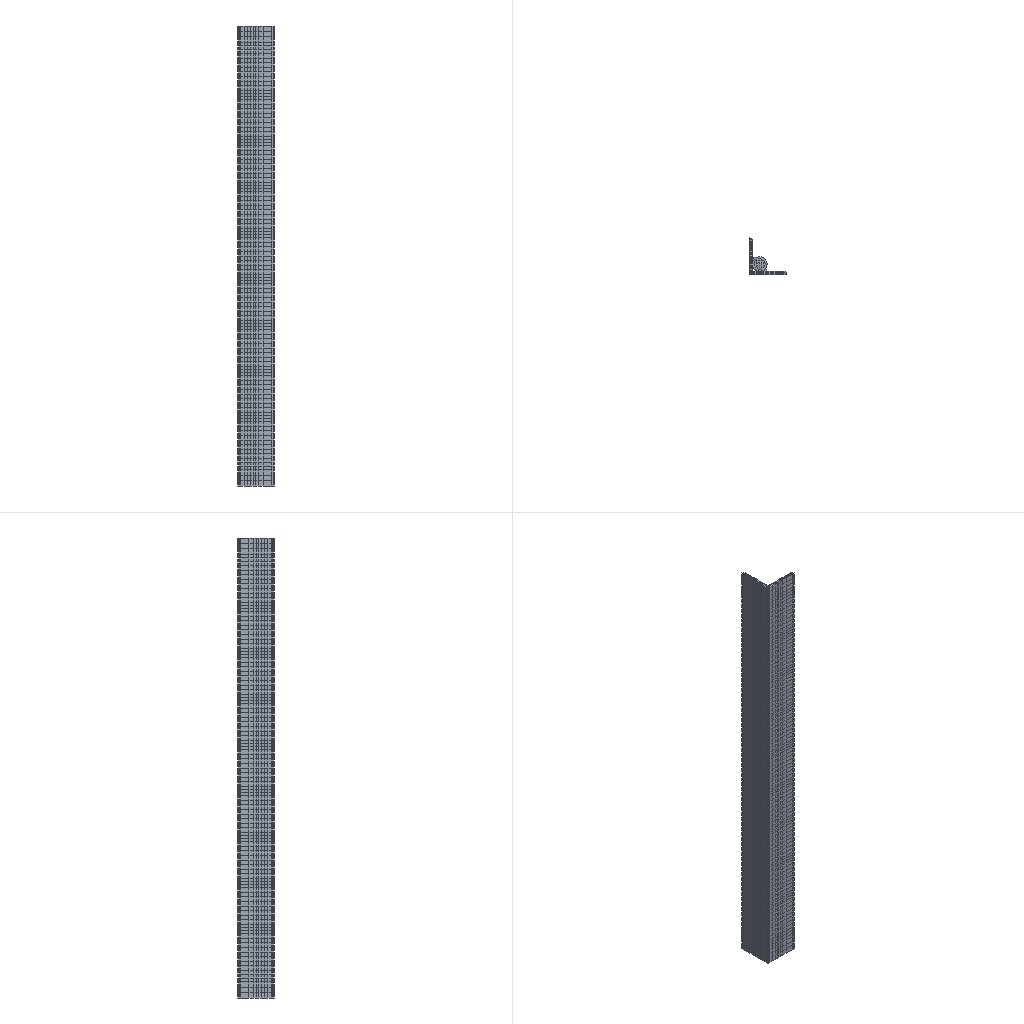Simulation study | abaqus
Set-up summary:
category,name,step,type,value,unit,region
solver,abaqus
solver,version,,,Abaqus/Explicit 3DEXPERIENCE R2017x
units,not stated in the deck,,not stated
analysis,deck,,transient,transient
load_step,Step-2,Step-2,transient
load_step,requested,,,1
mesh,nodes,,,15766
mesh,elements,,,12256
element_type,C3D8R,,solid,12256
load,load commands in deck,,count,1
bc,support commands in deck,,count,15
material,Q235,,in results
check,setup vs results,,match,"per instance, exact: element labels, types and connectivity; labels of the nodes the elements use; coordinates not compared"
Abaqus input file, long lists of numbers shortened:
*Heading
** Job name: Job-final Model name: yawan
** Generated by: Abaqus/CAE 2017
*Preprint, echo=NO, model=NO, history=NO, contact=NO
**
** PARTS
**
*Part, name=PART-1
*Node
      1, 0.002595, 0.005076, -0.36
      2, 0.002595, -0.0009244, -0.36
** (15764 more lines like these left out)
*Element, type=C3D8R
    1,   716,  4724, 11552,  4720,     1,   699,  4712,   706
    2,  4724,  4725, 11553, 11552,   699,   700,  4713,  4712
** (12254 more lines like these left out)
*Nset, nset=SET-T, generate
     1,  15766,      1
*Elset, elset=SET-T, generate
     1,  12256,      1
** Section: Section-1-SET-T
*Solid Section, elset=SET-T, material=Q235
,
*End Part
**
**
** ASSEMBLY
**
*Assembly, name=Assembly
**
*Instance, name=PART-1-1, part=PART-1
*End Instance
**
*Node
      1, 0.002795, 0.02128,          0.5
      2, 0.002795, 0.02128,         -0.5
*Nset, nset=Set-13
 2,
*Nset, nset=Set-14
 1,
*Elset, elset=Set-15, instance=PART-1-1, generate
     1,  12256,      1
*Nset, nset=Set-16, instance=PART-1-1, generate
     1,  15766,      1
*Nset, nset=Set-16
 1, 2
*Nset, nset=Set-17, instance=PART-1-1
     2,     3,     6,     7,    10,    11,    13,    16,   115,   116,   118,   119,   123,   124,   126,   127
   131,   132,   134,   137,   140,   141,   142,   145,   146,   149,   150,   153,   154,   156,   159,   162
** (94 more lines like these left out)
*Elset, elset=Set-22, instance=PART-1-1, generate
     1,  12256,      1
*Elset, elset=Set-23, instance=PART-1-1, generate
     1,  12256,      1
*Nset, nset=Set-24
 1,
*Nset, nset=Set-25
 1,
*Nset, nset=m_Set-17
 1,
*Nset, nset=m_Set-18
 2,
*Nset, nset=m_Set-19
 1,
*Nset, nset=m_Set-20
 2,
*Nset, nset=s_Set-20, instance=PART-1-1
   116,   117,   119,   120,   144,   145,   350,   351,   352,   353,   354,   355,   426,   427,   475,   476
   495,   496,   548,   549,   572,   657,  1088,  1089,  1096,  1097,  1100,  1102,  1182,  1183,  2346,  2351
** (4 more lines like these left out)
*Nset, nset=s_Set-21, instance=PART-1-1
   136,   137,   139,   140,   154,   155,   178,   179,   316,   317,   318,   319,   356,   357,   393,   394
   435,   436,   547,   570,   574,   658,  1162,  1163,  1170,  1171,  1174,  1176,  1214,  1215,  1282,  1283
** (4 more lines like these left out)
*Elset, elset=_SURF-1_S2, internal, instance=PART-1-1
 7817, 7818, 7819, 7820, 7821, 9959, 9960, 9961, 9962, 9963, 9964, 9965, 9966, 9967
*Elset, elset=_SURF-1_S3, internal, instance=PART-1-1
 8327, 8328, 8331
*Elset, elset=_SURF-1_S4, internal, instance=PART-1-1
 2524, 2527, 2530, 8325, 8326
*Elset, elset=_SURF-1_S5, internal, instance=PART-1-1
  457,  458,  459,  466,  467,  468,  559,  560,  561, 4244, 4245, 4246, 4253, 4254, 4255, 4262
 4263, 4264, 5003, 5004, 5005, 5012, 5013, 5014, 6077, 6078, 6079, 6086, 6087, 6088, 6095, 6096
** (1 more lines like these left out)
*Elset, elset=_SURF-1_S6, internal, instance=PART-1-1, generate
 2504,  2519,     3
*Elset, elset=_SURF-2_S2, internal, instance=PART-1-1, generate
 9986,  9994,     1
*Elset, elset=_SURF-2_S3, internal, instance=PART-1-1
 8295, 8300, 8301, 8337, 8338, 8343, 8345
*Elset, elset=_SURF-2_S4, internal, instance=PART-1-1
 8293, 8294, 8342
*Elset, elset=_SURF-2_S5, internal, instance=PART-1-1
  541,  542,  543,  550,  551,  552,  601,  602,  603,  694,  695,  696,  703,  704,  705,  712
  713,  714, 2645, 2646, 2647, 2654, 2655, 2656, 3455, 3456, 3457, 3464, 3465, 3466, 3473, 3474
** (1 more lines like these left out)
*Elset, elset=_SURF-2_S6, internal, instance=PART-1-1, generate
 2135,  2141,     3
*Elset, elset=_SURF-1_S5_1, internal, instance=PART-1-1
  457,  458,  459,  466,  467,  468,  559,  560,  561, 4244, 4245, 4246, 4253, 4254, 4255, 4262
 4263, 4264, 5003, 5004, 5005, 5012, 5013, 5014, 6077, 6078, 6079, 6086, 6087, 6088, 6095, 6096
** (1 more lines like these left out)
*Elset, elset=_SURF-1_S4_1, internal, instance=PART-1-1
 2524, 2527, 2530, 8325, 8326
*Elset, elset=_SURF-1_S6_1, internal, instance=PART-1-1, generate
 2504,  2519,     3
*Elset, elset=_SURF-1_S2_1, internal, instance=PART-1-1
 7817, 7818, 7819, 7820, 7821, 9959, 9960, 9961, 9962, 9963, 9964, 9965, 9966, 9967
*Elset, elset=_SURF-1_S3_1, internal, instance=PART-1-1
 8327, 8328, 8331
*Surface, type=ELEMENT, name=SURF-1
_SURF-1_S5_1, S5
_SURF-1_S4_1, S4
_SURF-1_S6_1, S6
_SURF-1_S2_1, S2
_SURF-1_S3_1, S3
*Elset, elset=_SURF-2_S5_1, internal, instance=PART-1-1
  541,  542,  543,  550,  551,  552,  601,  602,  603,  694,  695,  696,  703,  704,  705,  712
  713,  714, 2645, 2646, 2647, 2654, 2655, 2656, 3455, 3456, 3457, 3464, 3465, 3466, 3473, 3474
** (1 more lines like these left out)
*Elset, elset=_SURF-2_S6_1, internal, instance=PART-1-1, generate
 2135,  2141,     3
*Elset, elset=_SURF-2_S4_1, internal, instance=PART-1-1
 8293, 8294, 8342
*Elset, elset=_SURF-2_S2_1, internal, instance=PART-1-1, generate
 9986,  9994,     1
*Elset, elset=_SURF-2_S3_1, internal, instance=PART-1-1
 8295, 8300, 8301, 8337, 8338, 8343, 8345
*Surface, type=ELEMENT, name=SURF-2
_SURF-2_S5_1, S5
_SURF-2_S6_1, S6
_SURF-2_S4_1, S4
_SURF-2_S2_1, S2
_SURF-2_S3_1, S3
*Elset, elset=_Surf-3_S1, internal, instance=PART-1-1
 1254, 1255, 1256, 1257, 1435, 1436, 1437, 1438, 1439, 1440, 1441, 1442, 1443, 1444, 2141, 2142
 2143, 2176, 2177, 2178, 2179, 2180, 2181, 2182, 2183, 2184, 2185, 2186, 2187, 2188, 2189, 2190
** (11 more lines like these left out)
*Elset, elset=_Surf-3_S2, internal, instance=PART-1-1
   865,   866,   867,   868,   869,   870,   871,   872,   873,   874,   875,   876,  1036,  1037,  1038,  1039
  1040,  1041,  1076,  1077,  1078,  1079,  1084,  1085,  1086,  1087,  1088,  1089,  1090,  1091,  1092,  1093
** (35 more lines like these left out)
*Elset, elset=_Surf-3_S3, internal, instance=PART-1-1
   823,   824,   825,   832,   833,   834,   841,   842,   843,   873,   874,   893,   894,   897,   898,   928
   929,   932,   933,   952,   953,   954,   958,   959,   960,   976,   977,   980,   981,   984,   985,  1004
** (66 more lines like these left out)
*Elset, elset=_Surf-3_S4, internal, instance=PART-1-1
     3,     6,     9,    12,    15,    18,    21,    24,    27,    30,    33,    36,    39,    42,    45,    48
    51,    54,    57,    60,    63,    66,    69,    72,    75,    78,    81,    84,    87,    90,    93,    96
** (172 more lines like these left out)
*Elset, elset=_Surf-3_S5, internal, instance=PART-1-1
   457,   458,   459,   466,   467,   468,   541,   542,   543,   550,   551,   552,   559,   560,   561,   601
   602,   603,   694,   695,   696,   703,   704,   705,   712,   713,   714,   829,   830,   831,   838,   839
** (33 more lines like these left out)
*Elset, elset=_Surf-3_S6, internal, instance=PART-1-1
     1,     4,     7,    10,    13,    16,    19,    22,    25,    28,    31,    34,    37,    40,    43,    46
    49,    52,    55,    58,    61,    64,    67,    70,    73,    76,    79,    82,    85,    88,    91,    94
** (119 more lines like these left out)
*Surface, type=ELEMENT, name=Surf-3
_Surf-3_S1, S1
_Surf-3_S2, S2
_Surf-3_S4, S4
_Surf-3_S6, S6
_Surf-3_S3, S3
_Surf-3_S5, S5
*Elset, elset=_Surf-4_S1, internal, instance=PART-1-1
 1254, 1255, 1256, 1257, 1435, 1436, 1437, 1438, 1439, 1440, 1441, 1442, 1443, 1444, 2141, 2142
 2143, 2176, 2177, 2178, 2179, 2180, 2181, 2182, 2183, 2184, 2185, 2186, 2187, 2188, 2189, 2190
** (11 more lines like these left out)
*Elset, elset=_Surf-4_S2, internal, instance=PART-1-1
   865,   866,   867,   868,   869,   870,   871,   872,   873,   874,   875,   876,  1036,  1037,  1038,  1039
  1040,  1041,  1076,  1077,  1078,  1079,  1084,  1085,  1086,  1087,  1088,  1089,  1090,  1091,  1092,  1093
** (35 more lines like these left out)
*Elset, elset=_Surf-4_S3, internal, instance=PART-1-1
   823,   824,   825,   832,   833,   834,   841,   842,   843,   873,   874,   893,   894,   897,   898,   928
   929,   932,   933,   952,   953,   954,   958,   959,   960,   976,   977,   980,   981,   984,   985,  1004
** (66 more lines like these left out)
*Elset, elset=_Surf-4_S4, internal, instance=PART-1-1
     3,     6,     9,    12,    15,    18,    21,    24,    27,    30,    33,    36,    39,    42,    45,    48
    51,    54,    57,    60,    63,    66,    69,    72,    75,    78,    81,    84,    87,    90,    93,    96
** (172 more lines like these left out)
*Elset, elset=_Surf-4_S5, internal, instance=PART-1-1
   457,   458,   459,   466,   467,   468,   541,   542,   543,   550,   551,   552,   559,   560,   561,   601
   602,   603,   694,   695,   696,   703,   704,   705,   712,   713,   714,   829,   830,   831,   838,   839
** (33 more lines like these left out)
*Elset, elset=_Surf-4_S6, internal, instance=PART-1-1
     1,     4,     7,    10,    13,    16,    19,    22,    25,    28,    31,    34,    37,    40,    43,    46
    49,    52,    55,    58,    61,    64,    67,    70,    73,    76,    79,    82,    85,    88,    91,    94
** (119 more lines like these left out)
*Surface, type=ELEMENT, name=Surf-4
_Surf-4_S1, S1
_Surf-4_S2, S2
_Surf-4_S4, S4
_Surf-4_S6, S6
_Surf-4_S3, S3
_Surf-4_S5, S5
*Elset, elset=_Surf-9_S1, internal, instance=PART-1-1
 1254, 1255, 1256, 1257, 1435, 1436, 1437, 1438, 1439, 1440, 1441, 1442, 1443, 1444, 2141, 2142
 2143, 2176, 2177, 2178, 2179, 2180, 2181, 2182, 2183, 2184, 2185, 2186, 2187, 2188, 2189, 2190
** (11 more lines like these left out)
*Elset, elset=_Surf-9_S2, internal, instance=PART-1-1
   865,   866,   867,   868,   869,   870,   871,   872,   873,   874,   875,   876,  1036,  1037,  1038,  1039
  1040,  1041,  1076,  1077,  1078,  1079,  1084,  1085,  1086,  1087,  1088,  1089,  1090,  1091,  1092,  1093
** (35 more lines like these left out)
*Elset, elset=_Surf-9_S3, internal, instance=PART-1-1
   823,   824,   825,   832,   833,   834,   841,   842,   843,   873,   874,   893,   894,   897,   898,   928
   929,   932,   933,   952,   953,   954,   958,   959,   960,   976,   977,   980,   981,   984,   985,  1004
** (66 more lines like these left out)
*Elset, elset=_Surf-9_S4, internal, instance=PART-1-1
     3,     6,     9,    12,    15,    18,    21,    24,    27,    30,    33,    36,    39,    42,    45,    48
    51,    54,    57,    60,    63,    66,    69,    72,    75,    78,    81,    84,    87,    90,    93,    96
** (172 more lines like these left out)
*Elset, elset=_Surf-9_S5, internal, instance=PART-1-1
   457,   458,   459,   466,   467,   468,   541,   542,   543,   550,   551,   552,   559,   560,   561,   601
   602,   603,   694,   695,   696,   703,   704,   705,   712,   713,   714,   829,   830,   831,   838,   839
** (33 more lines like these left out)
*Elset, elset=_Surf-9_S6, internal, instance=PART-1-1
     1,     4,     7,    10,    13,    16,    19,    22,    25,    28,    31,    34,    37,    40,    43,    46
    49,    52,    55,    58,    61,    64,    67,    70,    73,    76,    79,    82,    85,    88,    91,    94
** (119 more lines like these left out)
*Surface, type=ELEMENT, name=Surf-9
_Surf-9_S1, S1
_Surf-9_S2, S2
_Surf-9_S4, S4
_Surf-9_S6, S6
_Surf-9_S3, S3
_Surf-9_S5, S5
*Elset, elset=_Surf-10_S1, internal, instance=PART-1-1
 1254, 1255, 1256, 1257, 1435, 1436, 1437, 1438, 1439, 1440, 1441, 1442, 1443, 1444, 2141, 2142
 2143, 2176, 2177, 2178, 2179, 2180, 2181, 2182, 2183, 2184, 2185, 2186, 2187, 2188, 2189, 2190
** (11 more lines like these left out)
*Elset, elset=_Surf-10_S2, internal, instance=PART-1-1
   865,   866,   867,   868,   869,   870,   871,   872,   873,   874,   875,   876,  1036,  1037,  1038,  1039
  1040,  1041,  1076,  1077,  1078,  1079,  1084,  1085,  1086,  1087,  1088,  1089,  1090,  1091,  1092,  1093
** (35 more lines like these left out)
*Elset, elset=_Surf-10_S3, internal, instance=PART-1-1
   823,   824,   825,   832,   833,   834,   841,   842,   843,   873,   874,   893,   894,   897,   898,   928
   929,   932,   933,   952,   953,   954,   958,   959,   960,   976,   977,   980,   981,   984,   985,  1004
** (66 more lines like these left out)
*Elset, elset=_Surf-10_S4, internal, instance=PART-1-1
     3,     6,     9,    12,    15,    18,    21,    24,    27,    30,    33,    36,    39,    42,    45,    48
    51,    54,    57,    60,    63,    66,    69,    72,    75,    78,    81,    84,    87,    90,    93,    96
** (172 more lines like these left out)
*Elset, elset=_Surf-10_S5, internal, instance=PART-1-1
   457,   458,   459,   466,   467,   468,   541,   542,   543,   550,   551,   552,   559,   560,   561,   601
   602,   603,   694,   695,   696,   703,   704,   705,   712,   713,   714,   829,   830,   831,   838,   839
** (33 more lines like these left out)
*Elset, elset=_Surf-10_S6, internal, instance=PART-1-1
     1,     4,     7,    10,    13,    16,    19,    22,    25,    28,    31,    34,    37,    40,    43,    46
    49,    52,    55,    58,    61,    64,    67,    70,    73,    76,    79,    82,    85,    88,    91,    94
** (119 more lines like these left out)
*Surface, type=ELEMENT, name=Surf-10
_Surf-10_S1, S1
_Surf-10_S2, S2
_Surf-10_S4, S4
_Surf-10_S6, S6
_Surf-10_S3, S3
_Surf-10_S5, S5
*Elset, elset=_s_Surf-5_S2, internal, instance=PART-1-1
 7817, 7818, 7819, 7820, 7821, 9959, 9960, 9961, 9962, 9963, 9964, 9965, 9966, 9967
*Elset, elset=_s_Surf-5_S3, internal, instance=PART-1-1
 8327, 8328, 8331
*Elset, elset=_s_Surf-5_S4, internal, instance=PART-1-1
 2524, 2527, 2530, 8325, 8326
*Elset, elset=_s_Surf-5_S5, internal, instance=PART-1-1
  457,  458,  459,  466,  467,  468,  559,  560,  561, 4244, 4245, 4246, 4253, 4254, 4255, 4262
 4263, 4264, 5003, 5004, 5005, 5012, 5013, 5014, 6077, 6078, 6079, 6086, 6087, 6088, 6095, 6096
** (1 more lines like these left out)
*Elset, elset=_s_Surf-5_S6, internal, instance=PART-1-1, generate
 2504,  2519,     3
*Surface, type=ELEMENT, name=s_Surf-5
_s_Surf-5_S2, S2
_s_Surf-5_S3, S3
_s_Surf-5_S4, S4
_s_Surf-5_S6, S6
_s_Surf-5_S5, S5
*Elset, elset=_s_Surf-6_S2, internal, instance=PART-1-1, generate
 9986,  9994,     1
*Elset, elset=_s_Surf-6_S3, internal, instance=PART-1-1
 8295, 8300, 8301, 8337, 8338, 8343, 8345
*Elset, elset=_s_Surf-6_S4, internal, instance=PART-1-1
 8293, 8294, 8342
*Elset, elset=_s_Surf-6_S5, internal, instance=PART-1-1
  541,  542,  543,  550,  551,  552,  601,  602,  603,  694,  695,  696,  703,  704,  705,  712
  713,  714, 2645, 2646, 2647, 2654, 2655, 2656, 3455, 3456, 3457, 3464, 3465, 3466, 3473, 3474
** (1 more lines like these left out)
*Elset, elset=_s_Surf-6_S6, internal, instance=PART-1-1, generate
 2135,  2141,     3
*Surface, type=ELEMENT, name=s_Surf-6
_s_Surf-6_S2, S2
_s_Surf-6_S3, S3
_s_Surf-6_S4, S4
_s_Surf-6_S6, S6
_s_Surf-6_S5, S5
*Elset, elset=_s_Surf-7_S2, internal, instance=PART-1-1
 7817, 7818, 7819, 7820, 7821, 9959, 9960, 9961, 9962, 9963, 9964, 9965, 9966, 9967
*Elset, elset=_s_Surf-7_S3, internal, instance=PART-1-1
 8327, 8328, 8331
*Elset, elset=_s_Surf-7_S4, internal, instance=PART-1-1
 2524, 2527, 2530, 8325, 8326
*Elset, elset=_s_Surf-7_S5, internal, instance=PART-1-1
  457,  458,  459,  466,  467,  468,  559,  560,  561, 4244, 4245, 4246, 4253, 4254, 4255, 4262
 4263, 4264, 5003, 5004, 5005, 5012, 5013, 5014, 6077, 6078, 6079, 6086, 6087, 6088, 6095, 6096
** (1 more lines like these left out)
*Elset, elset=_s_Surf-7_S6, internal, instance=PART-1-1, generate
 2504,  2519,     3
*Surface, type=ELEMENT, name=s_Surf-7
_s_Surf-7_S2, S2
_s_Surf-7_S3, S3
_s_Surf-7_S4, S4
_s_Surf-7_S6, S6
_s_Surf-7_S5, S5
*Elset, elset=_s_Surf-8_S2, internal, instance=PART-1-1, generate
 9986,  9994,     1
*Elset, elset=_s_Surf-8_S3, internal, instance=PART-1-1
 8295, 8300, 8301, 8337, 8338, 8343, 8345
*Elset, elset=_s_Surf-8_S4, internal, instance=PART-1-1
 8293, 8294, 8342
*Elset, elset=_s_Surf-8_S5, internal, instance=PART-1-1
  541,  542,  543,  550,  551,  552,  601,  602,  603,  694,  695,  696,  703,  704,  705,  712
  713,  714, 2645, 2646, 2647, 2654, 2655, 2656, 3455, 3456, 3457, 3464, 3465, 3466, 3473, 3474
** (1 more lines like these left out)
*Elset, elset=_s_Surf-8_S6, internal, instance=PART-1-1, generate
 2135,  2141,     3
*Surface, type=ELEMENT, name=s_Surf-8
_s_Surf-8_S2, S2
_s_Surf-8_S3, S3
_s_Surf-8_S4, S4
_s_Surf-8_S6, S6
_s_Surf-8_S5, S5
*Surface, type=NODE, name=s_Set-20_CNS_, internal
s_Set-20, 1.
*Surface, type=NODE, name=s_Set-21_CNS_, internal
s_Set-21, 1.
** Constraint: Constraint-3
*Coupling, constraint name=Constraint-3, ref node=m_Set-19, surface=s_Set-20_CNS_
*Kinematic
** Constraint: Constraint-4
*Coupling, constraint name=Constraint-4, ref node=m_Set-20, surface=s_Set-21_CNS_
*Kinematic
*End Assembly
**
** MATERIALS
**
*Material, name=Q235
*Conductivity
 50.,  20.
 47., 250.
 40., 500.
 27., 750.
 30.,1000.
 35.,1500.
140.,1700.
142.,2500.
*Density
7820.,  20.
7700., 250.
7610., 500.
7550., 750.
7490.,1000.
7350.,1500.
7300.,1700.
7090.,2500.
*Elastic
 2.05e+11, 0.28,  20.
 1.87e+11, 0.29, 250.
  1.5e+11, 0.31, 500.
    7e+10, 0.35, 750.
    2e+10,  0.4,1000.
    1e+08, 0.45,1500.
    1e+06, 0.48,1700.
    1e+06, 0.49,2500.
*Expansion
 1.1e-05,
*Plastic
 2.35e+08,0.
*Specific Heat
460.,  20.
480., 250.
530., 500.
675., 750.
670.,1000.
660.,1500.
780.,1700.
820.,2500.
**
** INTERACTION PROPERTIES
**
*Surface Interaction, name=IntProp-1
*Friction
 0.3,
*Surface Behavior, pressure-overclosure=HARD
**
** PHYSICAL CONSTANTS
**
*Physical Constants, absolute zero=-273., stefan boltzmann=5.67e-08
**
** BOUNDARY CONDITIONS
**
** Name: [REDACTED]
*Boundary
Set-14, 1, 1
Set-14, 2, 2
Set-14, 6, 6
** Name: [REDACTED]
*Boundary
Set-13, 1, 1
Set-13, 2, 2
Set-13, 3, 3
Set-13, 6, 6
**
** PREDEFINED FIELDS
**
** Name: Predefined Field-1   Type: Stress
*Initial Conditions, type=STRESS, file=D:/___________/______/______/_____.___________________
**
** INTERACTIONS
**
** Interaction: Int-1
*Contact, op=NEW
*Contact Inclusions, ALL EXTERIOR
*Contact Property Assignment
 ,  , IntProp-1
** ----------------------------------------------------------------
**
** STEP: Step-2
**
*Step, name=Step-2, nlgeom=YES
*Dynamic, Explicit
, 1.
*Bulk Viscosity
0.06, 1.2
**
** BOUNDARY CONDITIONS
**
** Name: [REDACTED] : Velocity/Angular velocity
*Boundary, op=NEW, type=VELOCITY
Set-25, 3, 3, -0.1
** Name: [REDACTED]
*Boundary, op=NEW
Set-14, 1, 1
Set-14, 2, 2
Set-14, 6, 6
** Name: [REDACTED]
*Boundary, op=NEW
Set-13, 1, 1
Set-13, 2, 2
Set-13, 3, 3
Set-13, 6, 6
**
** OUTPUT REQUESTS
**
*Restart, write, number interval=1, time marks=NO
**
** FIELD OUTPUT: F-Output-1
**
*Output, field, number interval=100
*Node Output
CF, RF, RM, U, V
*Element Output, directions=YES
E, LE, MISES, MISESMAX, NFORC, PE, PEEQ, PEEQMAX, PEMAG, S, SDEG
*Contact Output
CSDMG,
**
** HISTORY OUTPUT: H-Output-1
**
*Output, history, frequency=1
*Node Output, nset=Set-14
RF1, RF2, RF3, U1, U2, U3
*End Step
Results summary:
result,step,Step-2,partial,increments=442232 time=0.1266/1.0
result,analysis,,,transient
result,last_loadstep,,,1
result,primary field,,,U
result,reaction total,,FX,45.559,model units
result,reaction total,,FY,41.698,model units
result,reaction total,,FZ,4.539,model units